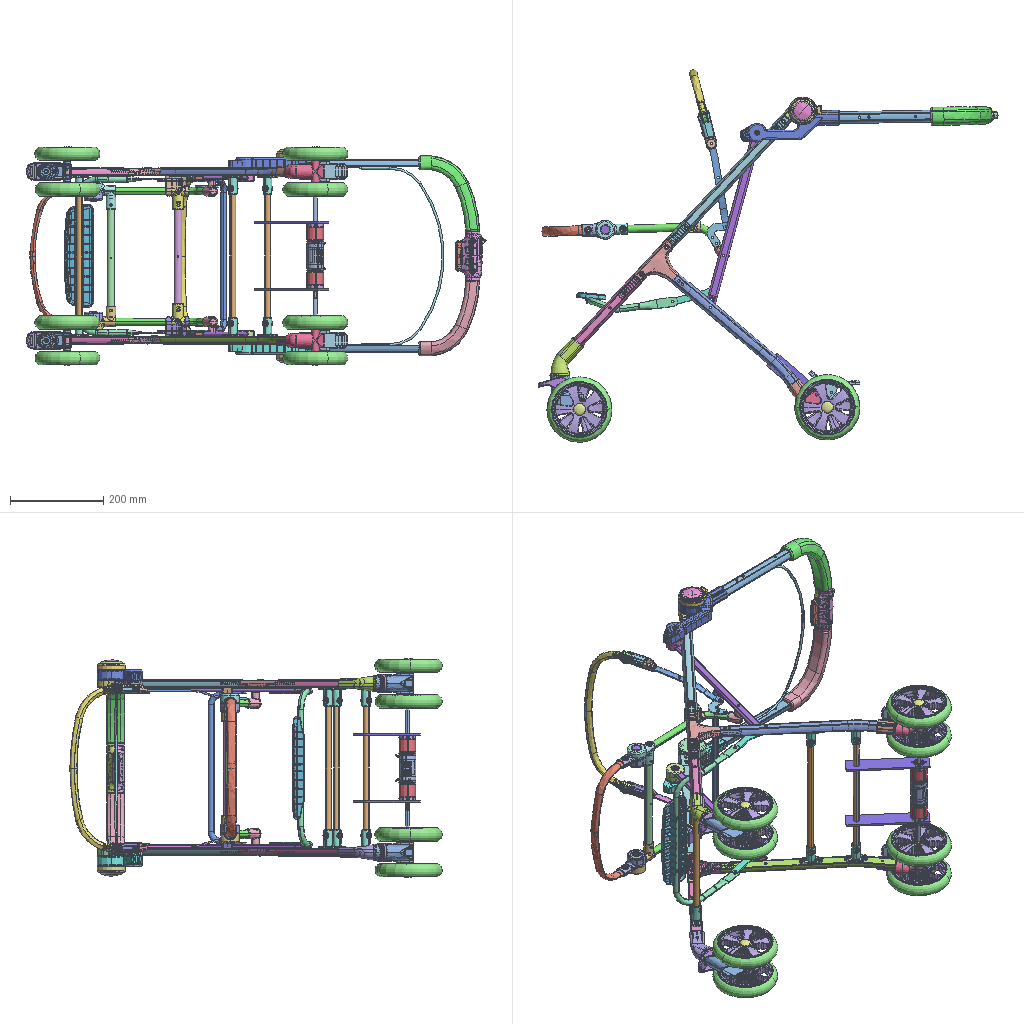Assembly | SolidWorks | 129 different items | 225 placed | box 985 x 797 x 469 mm
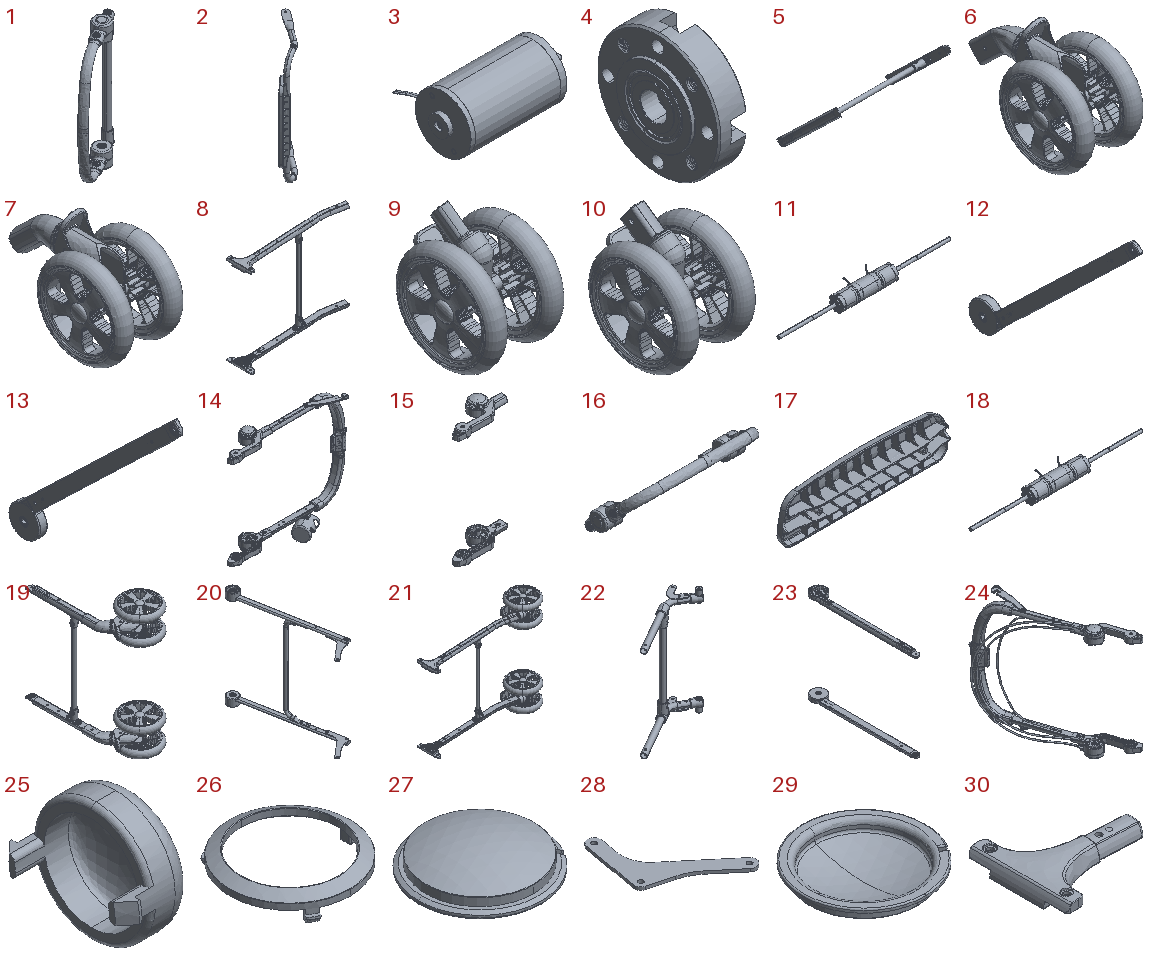Parts list (item | name | quantity | parent item | size | volume | features):
1 | (subassembly) | x1 | - | 166.776 x 106.592 x 321.08 mm | 136620 mm3 | -
2 | (subassembly) | x1 | - | 164.156 x 152.53 x 345 mm | 87735 mm3 | -
3 | (subassembly) | x2 | in 18 | 78 x 51.825 x 36 mm | 33870 mm3 | -
4 | (subassembly) | x2 | in 18 | 12.18 x 36 x 36 mm | 7699 mm3 | -
5 | (subassembly) | x1 | in 19 | 377 x 203.126 x 191.613 mm | 96779 mm3 | -
6 | (subassembly) | x1 | in 19 | 107.069 x 223.806 x 158.072 mm | 470883 mm3 | -
7 | (subassembly) | x1 | in 19 | 107.069 x 223.806 x 158.072 mm | 459720 mm3 | -
8 | (subassembly) | x1 | in 21 | 457.689 x 102.814 x 377.765 mm | 176220 mm3 | -
9 | (subassembly) | x1 | in 21 | 107.069 x 147.864 x 154.401 mm | 436546 mm3 | -
10 | (subassembly) | x1 | in 21 | 107.069 x 147.864 x 155.16 mm | 448012 mm3 | -
11 | (subassembly) | x1 | - | - | 142383 mm3 | -
12 | (subassembly) | x1 | in 23 | 16.903 x 352.818 x 314.841 mm | 72697 mm3 | -
13 | (subassembly) | x1 | in 23 | 16.903 x 328.024 x 340.536 mm | 72684 mm3 | -
14 | (subassembly) | x1 | in 24 | - | 680995 mm3 | -
15 | (subassembly) | x1 | in 14 | 212.741 x 95 x 464 mm | 193426 mm3 | -
16 | (subassembly) | x1 | in 1 | 321.08 x 143.863 x 138.826 mm | 126881 mm3 | -
17 | (subassembly) | x1 | in 2 | - | - | -
18 | (subassembly) | x1 | in 11 | - | 139903 mm3 | features ReferencePattern 12, MirrorCompFeat 1
19 | (subassembly) | x1 | - | - | 1026914 mm3 | -
20 | (subassembly) | x1 | - | 98.066 x 431.233 x 374.485 mm | 114494 mm3 | -
21 | (subassembly) | x1 | - | - | 1062049 mm3 | -
22 | (subassembly) | x1 | - | 245.155 x 130.528 x 328.07 mm | 82395 mm3 | -
23 | (subassembly) | x1 | - | 59.608 x 452.387 x 376.651 mm | 145181 mm3 | -
24 | (subassembly) | x1 | - | - | 744445 mm3 | -
25 | - | x8 | in 6, 7, 9, 10 | 16.535 x 26.8 x 24.4 mm | 2199 mm3 | features BaseBody 1
26 | - | x1 | in 15 | 53.3 x 51.8 x 10.109 mm | 2195 mm3 | features BaseBody 1
27 | - | x1 | in 15 | 47.34 x 47.34 x 9.8 mm | 4396 mm3 | features BaseBody 1
28 | - | x2 | in 20 | 87.081 x 112.72 x 3 mm | 7302 mm3 | features BaseBody 1
29 | - | x1 | in 15 | 47.34 x 47.34 x 9.8 mm | 4402 mm3 | features BaseBody 1
30 | - | x1 | in 8 | 115.648 x 102.814 x 16.383 mm | 42708 mm3 | features BaseBody 1
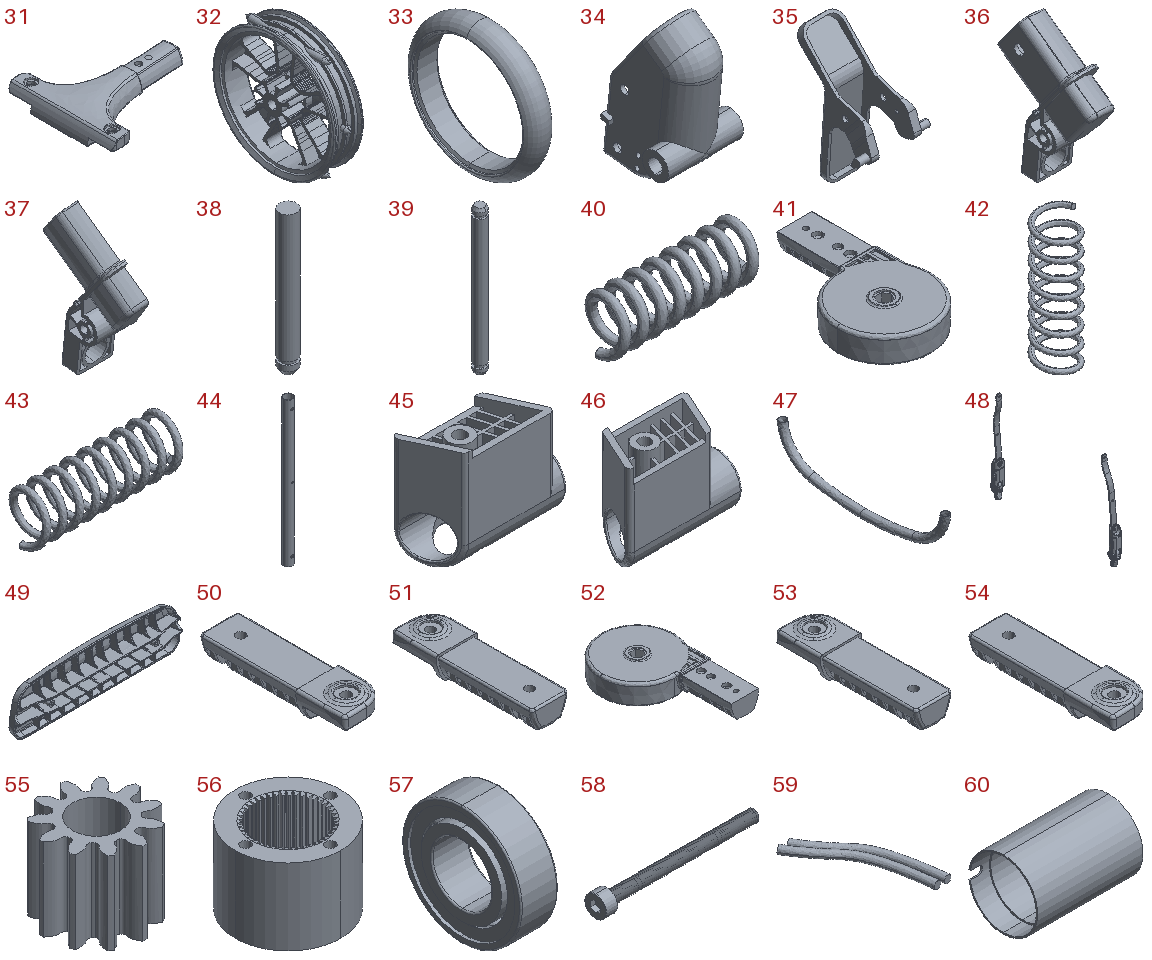31 | - | x1 | in 8 | 115.648 x 102.814 x 16.383 mm | 42837 mm3 | features BaseBody 1
32 | - | x8 | in 6, 7, 9, 10 | 29.19 x 122.462 x 117.58 mm | 68674 mm3 | features BaseBody 1, ICE 1
33 | - | x8 | in 6, 7, 9, 10 | 28.26 x 139.7 x 139.7 mm | 115471 mm3 | features BaseBody 1
34 | - | x2 | in 9, 10 | 46 x 53.095 x 84.854 mm | 26206 mm3 | features BaseBody 1
35 | - | x2 | in 9, 10 | 61.4 x 73.898 x 109.12 mm | 21040 mm3 | features BaseBody 1
36 | - | x1 | in 10 | 29.203 x 66.154 x 91.497 mm | 22564 mm3 | features BaseBody 1
37 | - | x1 | in 9 | 26.902 x 65.621 x 90.738 mm | 16180 mm3 | features BaseBody 1
38 | - | x1 | in 6 | 10 x 10 x 82 mm | 6302 mm3 | features BaseBody 1
39 | - | x2 | in 6, 10 | 8 x 8 x 98 mm | 4792 mm3 | features BaseBody 1
40 | - | x1 | in 6 | 17.991 x 6 x 6 mm | 99.073 mm3 | features BaseBody 1
41 | - | x1 | in 12 | 59.608 x 101.264 x 16.804 mm | 29040 mm3 | features BaseBody 1
42 | - | x1 | in 6 | 12.5 x 12.5 x 41.485 mm | 494.018 mm3 | features BaseBody 1
43 | - | x1 | in 9 | 37.488 x 11.5 x 11.5 mm | 503.734 mm3 | features BaseBody 1
44 | - | x1 | in 1 | 16 x 16 x 256 mm | 9739 mm3 | features BaseBody 1
45 | - | x1 | - | 51.079 x 21.892 x 44.191 mm | 16230 mm3 | features BaseBody 1
46 | - | x1 | - | 51.079 x 21.892 x 44.191 mm | 16196 mm3 | features BaseBody 1
47 | - | x1 | - | 16 x 356.5 x 92.983 mm | 16054 mm3 | features BaseBody 1
48 | - | x1 | - | 32.536 x 364.6 x 279.083 mm | 67490 mm3 | features BaseBody 10
49 | - | x1 | in 17 | - | - | features BaseBody 2, RefSurface 1
50 | - | x1 | in 12 | 24.436 x 81.569 x 16.763 mm | 14463 mm3 | features BaseBody 1
51 | - | x1 | in 5 | 24.436 x 81.569 x 16.763 mm | 14462 mm3 | features BaseBody 1
52 | - | x1 | in 13 | 59.608 x 101.264 x 16.804 mm | 29032 mm3 | features BaseBody 1
53 | - | x1 | in 13 | 24.436 x 81.569 x 16.763 mm | 14462 mm3 | features BaseBody 1
54 | - | x1 | in 5 | 24.436 x 81.569 x 16.763 mm | 14463 mm3 | features BaseBody 1
55 | - | x2 | in 18 | 6.47 x 6.407 x 5.5 mm | 81.586 mm3 | features BaseBody 1
56 | - | x2 | in 18 | 36 x 36 x 26 mm | 14714 mm3 | features BaseBody 1
57 | - | x4 | in 4 | 5 x 16 x 16 mm | 538.645 mm3 | features BaseBody 1
58 | - | x8 | in 18 | 41 x 5.5 x 5.5 mm | 259.671 mm3 | features BaseBody 1
59 | - | x2 | in 3 | 8.921 x 15.285 x 1 mm | 26.359 mm3 | features BaseBody 2
60 | - | x2 | in 3 | 55 x 36 x 36 mm | 8128 mm3 | features BaseBody 1
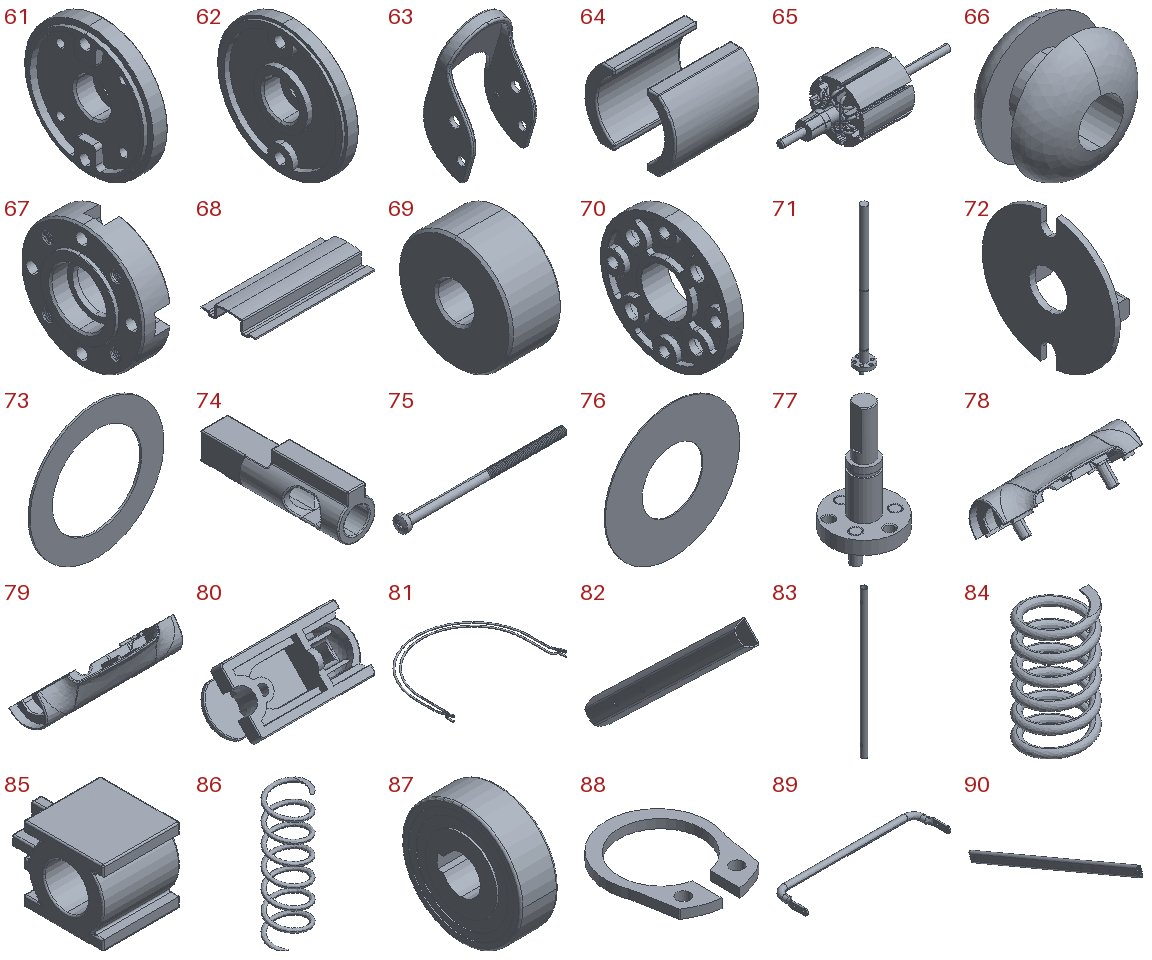61 | - | x2 | in 3 | 7.6 x 36 x 36 mm | 3322 mm3 | features BaseBody 1
62 | - | x2 | in 3 | 6.7 x 36 x 36 mm | 2836 mm3 | features BaseBody 1
63 | - | x2 | in 6, 7 | 39 x 29.721 x 73.171 mm | 8315 mm3 | features BaseBody 1
64 | - | x2 | in 3 | 30.643 x 33 x 25.929 mm | 7646 mm3 | features BaseBody 2
65 | - | x2 | in 3 | 76.5 x 24.777 x 24.8 mm | 8261 mm3 | features BaseBody 3
66 | - | x2 | in 3 | 8 x 6 x 8 mm | 125.45 mm3 | features BaseBody 1
67 | - | x2 | in 4 | 12 x 36 x 36 mm | 6610 mm3 | features BaseBody 1
68 | - | x4 | in 3 | 30.643 x 14.143 x 3.615 mm | 220.482 mm3 | features BaseBody 1
69 | - | x4 | in 3 | 4.5 x 10 x 10 mm | 315.579 mm3 | features BaseBody 1
70 | - | x2 | in 18 | 7.5 x 36 x 36 mm | 3397 mm3 | features BaseBody 1
71 | - | x2 | in 18 | 20.5 x 20.5 x 163.5 mm | 9096 mm3 | features ICE 2, BaseBody 1
72 | - | x2 | in 3 | 6.7 x 34.5 x 34.267 mm | 1641 mm3 | features BaseBody 3
73 | - | x2 | in 4 | 12 x 0.18 x 12 mm | 11.31 mm3 | features BaseBody 1
74 | - | x2 | in 6, 7 | 10.402 x 39.3 x 13 mm | 2086 mm3 | features BaseBody 1
75 | - | x4 | in 3 | 61.141 x 5.5 x 5.5 mm | 405.719 mm3 | features BaseBody 1
76 | - | x2 | in 18 | 22 x 0.18 x 22 mm | 54.287 mm3 | features BaseBody 1
77 | - | x1 | in 11 | 20.5 x 20.5 x 38.5 mm | 2479 mm3 | features BaseBody 1
78 | - | x1 | in 14 | 104.995 x 37.214 x 37.691 mm | 20077 mm3 | features BaseBody 1
79 | - | x1 | in 14 | 105 x 38.346 x 35.414 mm | 18588 mm3 | features BaseBody 1
80 | - | x1 | in 14 | 45.446 x 21.894 x 21.945 mm | 4020 mm3 | features BaseBody 1
81 | - | x1 | in 24 | 435.2 x 360.06 x 23.767 mm | 37382 mm3 | features BaseBody 2
82 | - | x2 | in 5 | 16 x 184.96 x 178.529 mm | 18508 mm3 | features BaseBody 1
83 | - | x3 | in 5, 8 | 13 x 13 x 343 mm | 15154 mm3 | features BaseBody 1
84 | - | x1 | in 7 | 12.495 x 12.5 x 23.645 mm | 403.779 mm3 | features BaseBody 1
85 | - | x2 | in 6, 7 | 15 x 20.5 x 14.5 mm | 2375 mm3 | features BaseBody 1
86 | - | x1 | in 7 | - | 32.094 mm3 | features BaseBody 1
87 | - | x2 | - | 7.854 x 24.97 x 24.99 mm | 3293 mm3 | features ICE 3, BaseBody 1, Scale 1
88 | - | x4 | in 18 | 8.901 x 10.834 x 0.774 mm | 24.698 mm3 | features BaseBody 1
89 | - | x1 | in 20 | 326 x 84 x 15.001 mm | 17967 mm3 | features BaseBody 1
90 | - | x2 | in 20 | 8 x 362.948 x 168.446 mm | 20758 mm3 | features BaseBody 1
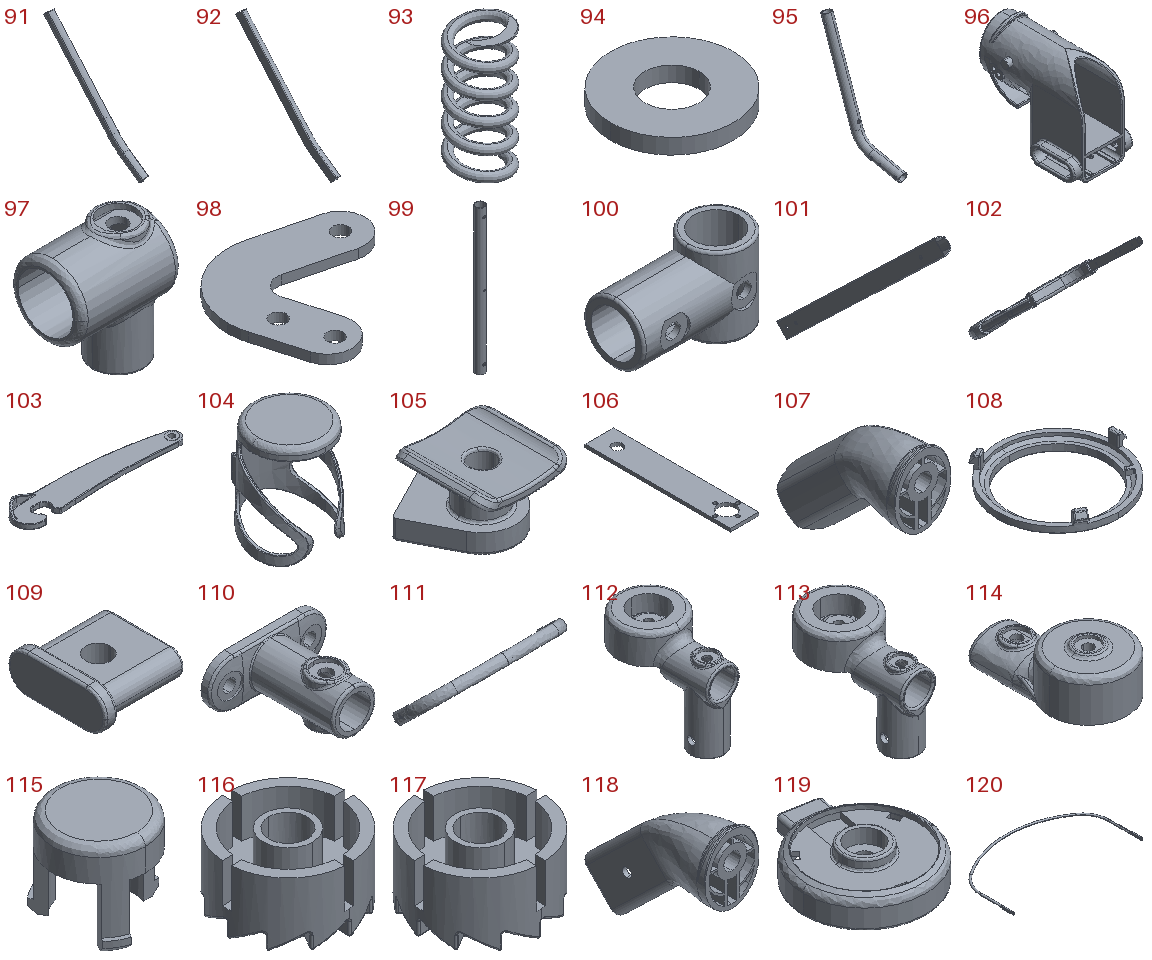91 | - | x1 | in 8 | 16 x 283.583 x 295.302 mm | 30959 mm3 | features BaseBody 1
92 | - | x1 | in 8 | 16 x 283.583 x 295.302 mm | 30931 mm3 | features BaseBody 1
93 | - | x1 | in 10 | 14 x 14 x 31.5 mm | 795.453 mm3 | features BaseBody 1
94 | - | x8 | in 2, 20 | 12.059 x 12.059 x 1.507 mm | 122.712 mm3 | features BaseBody 1
95 | - | x2 | in 22 | 16 x 149.335 x 206.465 mm | 14602 mm3 | features BaseBody 1
96 | - | x2 | in 6, 7 | 46 x 80.21 x 71.833 mm | 45997 mm3 | features BaseBody 1
97 | - | x2 | in 22 | 30 x 21.4 x 35.485 mm | 7040 mm3 | features BaseBody 1
98 | - | x2 | in 22 | 52.312 x 48.572 x 3 mm | 3515 mm3 | features BaseBody 1
99 | - | x1 | in 22 | 16 x 16 x 256 mm | 9739 mm3 | features BaseBody 1
100 | - | x2 | in 22 | 50.5 x 23 x 30.5 mm | 11175 mm3 | features BaseBody 1
101 | - | x2 | in 12, 13 | 16 x 280.261 x 269.738 mm | 29192 mm3 | features BaseBody 1
102 | - | x1 | in 14 | 428.555 x 285.247 x 274.529 mm | 356846 mm3 | features BaseBody 4
103 | - | x1 | in 14 | 148.137 x 27.348 x 12.258 mm | 8368 mm3 | features BaseBody 1
104 | - | x1 | in 14 | 69.285 x 75.31 x 89.558 mm | 30202 mm3 | features BaseBody 1
105 | - | x1 | in 14 | - | - | features BaseBody 1, FillRefSurface 1
106 | - | x2 | - | 35 x 180 x 4 mm | 22927 mm3 | features Extrusion 1, ICE 1
107 | - | x1 | in 7 | 33 x 80.996 x 71.706 mm | 27691 mm3 | features BaseBody 1
108 | - | x1 | in 15 | 53.3 x 51.8 x 10.109 mm | 2195 mm3 | features BaseBody 1
109 | - | x2 | in 20 | 17.5 x 20 x 8 mm | 1504 mm3 | features BaseBody 1
110 | - | x6 | in 5, 8 | 50 x 40 x 19.965 mm | 7929 mm3 | features BaseBody 1
111 | - | x1 | in 16 | 297.02 x 94.548 x 91.608 mm | 24402 mm3 | features BaseBody 1
112 | - | x1 | in 16 | 40 x 68.161 x 58.5 mm | 24836 mm3 | features BaseBody 1
113 | - | x1 | in 16 | 40 x 68.161 x 52.5 mm | 24103 mm3 | features BaseBody 1
114 | - | x2 | in 16 | 40 x 70 x 34 mm | 17065 mm3 | features BaseBody 1
115 | - | x2 | in 16 | 23.2 x 23.006 x 21.7 mm | 2251 mm3 | features BaseBody 1
116 | - | x1 | in 16 | 34.702 x 34.702 x 21.496 mm | 7230 mm3 | features BaseBody 1
117 | - | x1 | in 16 | 34.702 x 34.702 x 21.496 mm | 7311 mm3 | features BaseBody 1
118 | - | x1 | in 6 | 33 x 80.996 x 71.706 mm | 27661 mm3 | features BaseBody 1
119 | - | x2 | in 24 | 60 x 70.94 x 18.527 mm | 21713 mm3 | features BaseBody 1
120 | - | x1 | in 24 | 384 x 214.497 x 8 mm | 13043 mm3 | features BaseBody 1
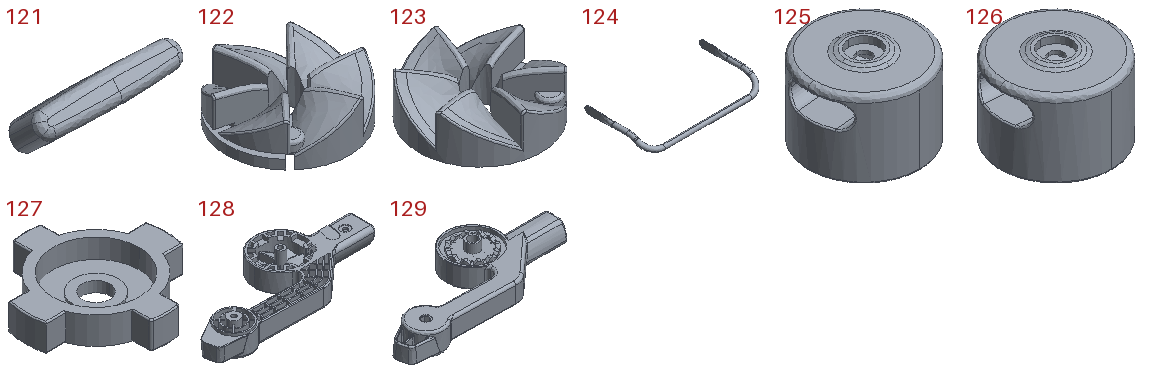121 | - | x1 | in 14 | 65.6 x 38.87 x 37.679 mm | 10434 mm3 | features BaseBody 1
122 | - | x1 | in 14 | 40.118 x 40.118 x 13.737 mm | 8402 mm3 | features BaseBody 1
123 | - | x1 | in 14 | 40.118 x 40.118 x 13.737 mm | 8419 mm3 | features BaseBody 1
124 | - | x1 | in 2 | 342 x 189.784 x 41.985 mm | 25902 mm3 | features BaseBody 1
125 | - | x1 | in 20 | 40 x 40 x 27.99 mm | 18357 mm3 | features BaseBody 1
126 | - | x1 | in 20 | 40 x 40 x 27.99 mm | 18359 mm3 | features BaseBody 1
127 | - | x2 | in 14 | 53.657 x 53.657 x 10.33 mm | 10160 mm3 | features BaseBody 1
128 | - | x1 | in 15 | 212.741 x 95 x 36 mm | 90575 mm3 | features BaseBody 1
129 | - | x1 | in 15 | 212.741 x 95 x 36 mm | 90417 mm3 | features BaseBody 1
Mates (type | each side: item.copy, entity, surface, feature):
Concentric | 30.1 face cylinder Input 1 | 51.1 face cylinder Input 1
Concentric | 30.1 face cylinder Input 1 | 50.1 face cylinder Input 1
DistanceDim | 50.1 face plane Input 1 | 30.1 face plane Input 1
Concentric | 82.1 face cylinder Input 1 | 94.1 face cylinder Input 1
DistanceDim | 94.1 face plane Input 1 | 82.1 face plane Input 1
DistanceDim | 124.1 face plane Input 1 | 28.1 face plane Input 1
Concentric | 28.1 face cylinder Input 1 | 124.1 face cylinder Input 1
Concentric | 90.1 face cylinder Input 1 | 97.1 face cylinder Input 1
DistanceDim | 90.1 face plane Input 1 | 98.1 face plane Input 1
Concentric | 98.1 face cylinder Input 1 | 48.1 face cylinder Input 4
DistanceDim | 48.1 face plane Input 4 | 98.1 face plane Input 1
Concentric | 48.1 face cylinder Input 3 | 47.1 face cylinder Input 1
Lock | 48.1 select_type:0 | 47.1 select_type:0
Concentric | 95.1 face cylinder Input 1 | 113.1 face cylinder Input 1 | 2 times
Concentric | 46.1 face cylinder Input 1 | 95.2 face cylinder Input 1
DistanceDim | 51.1 face plane Input 1 | 30.1 face plane Input 1
Concentric | 45.1 face cylinder Input 1 | 95.1 face cylinder Input 1
Concentric | 41.1 face cone Input 2 | 128.1 face cylinder Input 1
Concentric | 128.1 face cylinder Input 1 | 125.1 face cylinder Input 1
Concentric | 50.1 face cylinder Input 1 | 45.1 face cylinder Input 1
Concentric | 53.1 face cylinder Input 1 | 46.1 face cylinder Input 1
Coincident | 41.1 face plane Input 2 | 128.1 face plane Input 1
Tangent | 33.1 face torus Input 1 | assembly plane
Parallel | 92.1 face plane Input 1 | assembly plane
Concentric | 34.1 face cylinder Input 1 | 56.1 face cylinder Input 1
Concentric | 32.1 face cylinder Input 1 | 87.1 face cylinder Input 1
Coincident | 32.1 face plane Cut-Extrude1 | 87.1 face plane Input 1
Width | 35.1 face plane Input 1 | 35.2 face plane Input 1 | 67.1 face plane Input 1 | 67.2 face plane Input 1
Concentric | 32.2 face cylinder Input 1 | 87.2 face cylinder Boss-Extrude1
Coincident | 32.2 face plane Cut-Extrude1 | 87.2 face plane Input 1
Concentric | 110.1 face cylinder Input 1 | 83.1 face cylinder Input 1 | 2 times
Concentric | 83.1 face cylinder Input 1 | 110.2 face cylinder Input 1
Coincident | 92.1 face plane Input 1 | 110.2 face plane Input 1
Parallel | 110.3 face plane Input 1 | 110.2 face plane Input 1
Coincident | 110.3 face plane Input 1 | 110.2 face plane Input 1
Concentric | 83.1 face cylinder Input 1 | 106.1 face cylinder Boss-Extrude1
Concentric | 60.1 face cylinder Input 1 | 106.1 face cylinder Boss-Extrude1
Concentric | 67.2 face cylinder Input 1 | 106.1 face cylinder Cut-Extrude2
Coincident | 67.2 face plane Input 1 | 106.1 face plane Boss-Extrude1
Concentric | 83.1 face cylinder Input 1 | 106.2 face cylinder Boss-Extrude1
Concentric | 67.1 face cylinder Input 1 | 106.2 face cylinder Boss-Extrude1
Coincident | 67.1 face plane Input 1 | 106.2 face plane Boss-Extrude1
Concentric | 71.1 face cylinder Cut-Extrude1 | 88.1 face cylinder Input 1
Coincident | 87.1 face plane Input 1 | 88.1 face plane Input 1
Concentric | 71.2 face cylinder Input 1 | 88.2 face cylinder Input 1
Coincident | 87.2 face plane Input 1 | 88.2 face plane Input 1
Parallel | 31.1 face cylinder Input 1 | 82.2 face cylinder Input 1
Parallel | 31.1 face cylinder Input 1 | 101.1 face cylinder Input 1